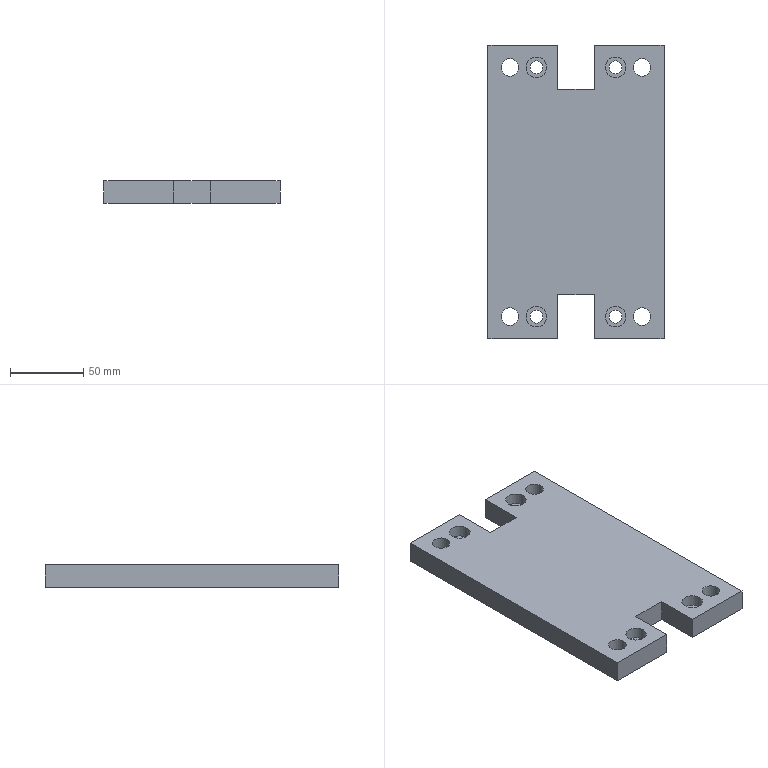Part | STEP file | 冲床-300配套压波_id854_x_t | 1 solid | 30 faces | box 120 x 200 x 15 mm | volume 324088 mm3 | plane 18 | cylinder 12 | commonest cylinder face diameters 8.7 x4 12 x4 14 x4
STEP:
#1=CARTESIAN_POINT('',(1785.,85.,60.));
#2=VERTEX_POINT('',#1);
#3=CARTESIAN_POINT('',(1778.,85.,60.));
#4=DIRECTION('',(0.,0.,-1.));
#5=DIRECTION('',(1.,0.,0.));
#6=AXIS2_PLACEMENT_3D('',#3,#4,#5);
#7=CIRCLE('',#6,7.);
#8=EDGE_CURVE('',#2,#2,#7,.T.);
#9=ORIENTED_EDGE('',*,*,#8,.F.);
#10=EDGE_LOOP('',(#9));
#11=FACE_BOUND('',#10,.T.);
#12=CARTESIAN_POINT('',(1782.35,85.,60.));
#13=VERTEX_POINT('',#12);
#14=CARTESIAN_POINT('',(1778.,85.,60.));
#15=DIRECTION('',(0.,0.,-1.));
#16=DIRECTION('',(1.,0.,0.));
#17=AXIS2_PLACEMENT_3D('',#14,#15,#16);
#18=CIRCLE('',#17,4.35);
#19=EDGE_CURVE('',#13,#13,#18,.T.);
#20=ORIENTED_EDGE('',*,*,#19,.T.);
#21=EDGE_LOOP('',(#20));
#22=FACE_BOUND('',#21,.T.);
#23=CARTESIAN_POINT('',(1778.,85.,60.));
#24=DIRECTION('',(0.,0.,1.));
#25=DIRECTION('',(1.,0.,0.));
#26=AXIS2_PLACEMENT_3D('',#23,#24,#25);
#27=PLANE('',#26);
#28=ADVANCED_FACE('',(#11,#22),#27,.T.);
#29=CARTESIAN_POINT('',(1782.35,85.,53.));
#30=VERTEX_POINT('',#29);
#31=CARTESIAN_POINT('',(1778.,85.,53.));
#32=DIRECTION('',(0.,0.,1.));
#33=DIRECTION('',(1.,0.,0.));
#34=AXIS2_PLACEMENT_3D('',#31,#32,#33);
#35=CIRCLE('',#34,4.35);
#36=EDGE_CURVE('',#30,#30,#35,.T.);
#37=ORIENTED_EDGE('',*,*,#36,.F.);
#38=EDGE_LOOP('',(#37));
#39=FACE_BOUND('',#38,.T.);
#40=ORIENTED_EDGE('',*,*,#19,.F.);
#41=EDGE_LOOP('',(#40));
#42=FACE_BOUND('',#41,.T.);
#43=CARTESIAN_POINT('',(1778.,85.,87.));
#44=DIRECTION('',(0.,0.,-1.));
#45=DIRECTION('',(-1.,0.,0.));
#46=AXIS2_PLACEMENT_3D('',#43,#44,#45);
#47=CYLINDRICAL_SURFACE('',#46,4.35);
#48=ADVANCED_FACE('',(#39,#42),#47,.F.);
#49=ORIENTED_EDGE('',*,*,#8,.T.);
#50=EDGE_LOOP('',(#49));
#51=FACE_BOUND('',#50,.T.);
#52=CARTESIAN_POINT('',(1785.,85.,68.));
#53=VERTEX_POINT('',#52);
#54=CARTESIAN_POINT('',(1778.,85.,68.));
#55=DIRECTION('',(0.,0.,-1.));
#56=DIRECTION('',(1.,0.,0.));
#57=AXIS2_PLACEMENT_3D('',#54,#55,#56);
#58=CIRCLE('',#57,7.);
#59=EDGE_CURVE('',#53,#53,#58,.T.);
#60=ORIENTED_EDGE('',*,*,#59,.F.);
#61=EDGE_LOOP('',(#60));
#62=FACE_BOUND('',#61,.T.);
#63=CARTESIAN_POINT('',(1778.,85.,60.));
#64=DIRECTION('',(0.,0.,1.));
#65=DIRECTION('',(1.,0.,0.));
#66=AXIS2_PLACEMENT_3D('',#63,#64,#65);
#67=CYLINDRICAL_SURFACE('',#66,7.);
#68=ADVANCED_FACE('',(#51,#62),#67,.F.);
#69=CARTESIAN_POINT('',(1785.,-85.,60.));
#70=VERTEX_POINT('',#69);
#71=CARTESIAN_POINT('',(1778.,-85.,60.));
#72=DIRECTION('',(0.,0.,-1.));
#73=DIRECTION('',(1.,0.,0.));
#74=AXIS2_PLACEMENT_3D('',#71,#72,#73);
#75=CIRCLE('',#74,7.);
#76=EDGE_CURVE('',#70,#70,#75,.T.);
#77=ORIENTED_EDGE('',*,*,#76,.F.);
#78=EDGE_LOOP('',(#77));
#79=FACE_BOUND('',#78,.T.);
#80=CARTESIAN_POINT('',(1782.35,-85.,60.));
#81=VERTEX_POINT('',#80);
#82=CARTESIAN_POINT('',(1778.,-85.,60.));
#83=DIRECTION('',(0.,0.,-1.));
#84=DIRECTION('',(1.,0.,0.));
#85=AXIS2_PLACEMENT_3D('',#82,#83,#84);
#86=CIRCLE('',#85,4.35);
#87=EDGE_CURVE('',#81,#81,#86,.T.);
#88=ORIENTED_EDGE('',*,*,#87,.T.);
#89=EDGE_LOOP('',(#88));
#90=FACE_BOUND('',#89,.T.);
#91=CARTESIAN_POINT('',(1778.,-85.,60.));
#92=DIRECTION('',(0.,0.,1.));
#93=DIRECTION('',(1.,0.,0.));
#94=AXIS2_PLACEMENT_3D('',#91,#92,#93);
#95=PLANE('',#94);
#96=ADVANCED_FACE('',(#79,#90),#95,.T.);
#97=CARTESIAN_POINT('',(1825.,-85.,60.));
#98=VERTEX_POINT('',#97);
#99=CARTESIAN_POINT('',(1832.,-85.,60.));
#100=DIRECTION('',(0.,0.,-1.));
#101=DIRECTION('',(-1.,0.,0.));
#102=AXIS2_PLACEMENT_3D('',#99,#100,#101);
#103=CIRCLE('',#102,7.);
#104=EDGE_CURVE('',#98,#98,#103,.T.);
#105=ORIENTED_EDGE('',*,*,#104,.F.);
#106=EDGE_LOOP('',(#105));
#107=FACE_BOUND('',#106,.T.);
#108=CARTESIAN_POINT('',(1827.65,-85.,60.));
#109=VERTEX_POINT('',#108);
#110=CARTESIAN_POINT('',(1832.,-85.,60.));
#111=DIRECTION('',(0.,0.,-1.));
#112=DIRECTION('',(-1.,0.,0.));
#113=AXIS2_PLACEMENT_3D('',#110,#111,#112);
#114=CIRCLE('',#113,4.35);
#115=EDGE_CURVE('',#109,#109,#114,.T.);
#116=ORIENTED_EDGE('',*,*,#115,.T.);
#117=EDGE_LOOP('',(#116));
#118=FACE_BOUND('',#117,.T.);
#119=CARTESIAN_POINT('',(1832.,-85.,60.));
#120=DIRECTION('',(0.,0.,1.));
#121=DIRECTION('',(-1.,0.,0.));
#122=AXIS2_PLACEMENT_3D('',#119,#120,#121);
#123=PLANE('',#122);
#124=ADVANCED_FACE('',(#107,#118),#123,.T.);
#125=CARTESIAN_POINT('',(1856.,-85.,68.));
#126=VERTEX_POINT('',#125);
#127=CARTESIAN_POINT('',(1850.,-85.,68.));
#128=DIRECTION('',(0.,0.,1.));
#129=DIRECTION('',(1.,0.,0.));
#130=AXIS2_PLACEMENT_3D('',#127,#128,#129);
#131=CIRCLE('',#130,6.);
#132=EDGE_CURVE('',#126,#126,#131,.T.);
#133=ORIENTED_EDGE('',*,*,#132,.T.);
#134=EDGE_LOOP('',(#133));
#135=FACE_BOUND('',#134,.T.);
#136=CARTESIAN_POINT('',(1856.,-85.,53.));
#137=VERTEX_POINT('',#136);
#138=CARTESIAN_POINT('',(1850.,-85.,53.));
#139=DIRECTION('',(0.,0.,1.));
#140=DIRECTION('',(1.,0.,0.));
#141=AXIS2_PLACEMENT_3D('',#138,#139,#140);
#142=CIRCLE('',#141,6.);
#143=EDGE_CURVE('',#137,#137,#142,.T.);
#144=ORIENTED_EDGE('',*,*,#143,.F.);
#145=EDGE_LOOP('',(#144));
#146=FACE_BOUND('',#145,.T.);
#147=CARTESIAN_POINT('',(1850.,-85.,-78.5));
#148=DIRECTION('',(0.,0.,1.));
#149=DIRECTION('',(1.,0.,0.));
#150=AXIS2_PLACEMENT_3D('',#147,#148,#149);
#151=CYLINDRICAL_SURFACE('',#150,6.);
#152=ADVANCED_FACE('',(#135,#146),#151,.F.);
#153=CARTESIAN_POINT('',(1766.,-85.,68.));
#154=VERTEX_POINT('',#153);
#155=CARTESIAN_POINT('',(1760.,-85.,68.));
#156=DIRECTION('',(0.,0.,1.));
#157=DIRECTION('',(1.,0.,0.));
#158=AXIS2_PLACEMENT_3D('',#155,#156,#157);
#159=CIRCLE('',#158,6.);
#160=EDGE_CURVE('',#154,#154,#159,.T.);
#161=ORIENTED_EDGE('',*,*,#160,.T.);
#162=EDGE_LOOP('',(#161));
#163=FACE_BOUND('',#162,.T.);
#164=CARTESIAN_POINT('',(1766.,-85.,53.));
#165=VERTEX_POINT('',#164);
#166=CARTESIAN_POINT('',(1760.,-85.,53.));
#167=DIRECTION('',(0.,0.,1.));
#168=DIRECTION('',(1.,0.,0.));
#169=AXIS2_PLACEMENT_3D('',#166,#167,#168);
#170=CIRCLE('',#169,6.);
#171=EDGE_CURVE('',#165,#165,#170,.T.);
#172=ORIENTED_EDGE('',*,*,#171,.F.);
#173=EDGE_LOOP('',(#172));
#174=FACE_BOUND('',#173,.T.);
#175=CARTESIAN_POINT('',(1760.,-85.,-78.5));
#176=DIRECTION('',(0.,0.,1.));
#177=DIRECTION('',(1.,0.,0.));
#178=AXIS2_PLACEMENT_3D('',#175,#176,#177);
#179=CYLINDRICAL_SURFACE('',#178,6.);
#180=ADVANCED_FACE('',(#163,#174),#179,.F.);
#181=CARTESIAN_POINT('',(1856.,85.,68.));
#182=VERTEX_POINT('',#181);
#183=CARTESIAN_POINT('',(1850.,85.,68.));
#184=DIRECTION('',(0.,0.,1.));
#185=DIRECTION('',(1.,0.,0.));
#186=AXIS2_PLACEMENT_3D('',#183,#184,#185);
#187=CIRCLE('',#186,6.);
#188=EDGE_CURVE('',#182,#182,#187,.T.);
#189=ORIENTED_EDGE('',*,*,#188,.T.);
#190=EDGE_LOOP('',(#189));
#191=FACE_BOUND('',#190,.T.);
#192=CARTESIAN_POINT('',(1856.,85.,53.));
#193=VERTEX_POINT('',#192);
#194=CARTESIAN_POINT('',(1850.,85.,53.));
#195=DIRECTION('',(0.,0.,1.));
#196=DIRECTION('',(1.,0.,0.));
#197=AXIS2_PLACEMENT_3D('',#194,#195,#196);
#198=CIRCLE('',#197,6.);
#199=EDGE_CURVE('',#193,#193,#198,.T.);
#200=ORIENTED_EDGE('',*,*,#199,.F.);
#201=EDGE_LOOP('',(#200));
#202=FACE_BOUND('',#201,.T.);
#203=CARTESIAN_POINT('',(1850.,85.,-78.5));
#204=DIRECTION('',(0.,0.,1.));
#205=DIRECTION('',(1.,0.,0.));
#206=AXIS2_PLACEMENT_3D('',#203,#204,#205);
#207=CYLINDRICAL_SURFACE('',#206,6.);
#208=ADVANCED_FACE('',(#191,#202),#207,.F.);
#209=CARTESIAN_POINT('',(1766.,85.,68.));
#210=VERTEX_POINT('',#209);
#211=CARTESIAN_POINT('',(1760.,85.,68.));
#212=DIRECTION('',(0.,0.,1.));
#213=DIRECTION('',(1.,0.,0.));
#214=AXIS2_PLACEMENT_3D('',#211,#212,#213);
#215=CIRCLE('',#214,6.);
#216=EDGE_CURVE('',#210,#210,#215,.T.);
#217=ORIENTED_EDGE('',*,*,#216,.T.);
#218=EDGE_LOOP('',(#217));
#219=FACE_BOUND('',#218,.T.);
#220=CARTESIAN_POINT('',(1766.,85.,53.));
#221=VERTEX_POINT('',#220);
#222=CARTESIAN_POINT('',(1760.,85.,53.));
#223=DIRECTION('',(0.,0.,1.));
#224=DIRECTION('',(1.,0.,0.));
#225=AXIS2_PLACEMENT_3D('',#222,#223,#224);
#226=CIRCLE('',#225,6.);
#227=EDGE_CURVE('',#221,#221,#226,.T.);
#228=ORIENTED_EDGE('',*,*,#227,.F.);
#229=EDGE_LOOP('',(#228));
#230=FACE_BOUND('',#229,.T.);
#231=CARTESIAN_POINT('',(1760.,85.,-78.5));
#232=DIRECTION('',(0.,0.,1.));
#233=DIRECTION('',(1.,0.,0.));
#234=AXIS2_PLACEMENT_3D('',#231,#232,#233);
#235=CYLINDRICAL_SURFACE('',#234,6.);
#236=ADVANCED_FACE('',(#219,#230),#235,.F.);
#237=CARTESIAN_POINT('',(1817.52,70.,68.));
#238=VERTEX_POINT('',#237);
#239=CARTESIAN_POINT('',(1817.52,70.,53.));
#240=VERTEX_POINT('',#239);
#241=CARTESIAN_POINT('',(1817.52,70.,68.));
#242=DIRECTION('',(0.,0.,-1.));
#243=VECTOR('',#242,1.);
#244=LINE('',#241,#243);
#245=EDGE_CURVE('',#238,#240,#244,.T.);
#246=ORIENTED_EDGE('',*,*,#245,.F.);
#247=CARTESIAN_POINT('',(1817.52,100.,68.));
#248=VERTEX_POINT('',#247);
#249=CARTESIAN_POINT('',(1817.52,58.462,68.));
#250=DIRECTION('',(0.,1.,0.));
#251=VECTOR('',#250,1.);
#252=LINE('',#249,#251);
#253=EDGE_CURVE('',#238,#248,#252,.T.);
#254=ORIENTED_EDGE('',*,*,#253,.T.);
#255=CARTESIAN_POINT('',(1817.52,100.,53.));
#256=VERTEX_POINT('',#255);
#257=CARTESIAN_POINT('',(1817.52,100.,68.));
#258=DIRECTION('',(0.,0.,-1.));
#259=VECTOR('',#258,1.);
#260=LINE('',#257,#259);
#261=EDGE_CURVE('',#248,#256,#260,.T.);
#262=ORIENTED_EDGE('',*,*,#261,.T.);
#263=CARTESIAN_POINT('',(1817.52,58.462,53.));
#264=DIRECTION('',(0.,1.,0.));
#265=VECTOR('',#264,1.);
#266=LINE('',#263,#265);
#267=EDGE_CURVE('',#240,#256,#266,.T.);
#268=ORIENTED_EDGE('',*,*,#267,.F.);
#269=EDGE_LOOP('',(#246,#254,#262,#268));
#270=FACE_OUTER_BOUND('',#269,.T.);
#271=CARTESIAN_POINT('',(1817.52,58.462,68.));
#272=DIRECTION('',(-1.,0.,0.));
#273=DIRECTION('',(0.,0.,1.));
#274=AXIS2_PLACEMENT_3D('',#271,#272,#273);
#275=PLANE('',#274);
#276=ADVANCED_FACE('',(#270),#275,.T.);
#277=CARTESIAN_POINT('',(1792.48,70.,53.));
#278=VERTEX_POINT('',#277);
#279=CARTESIAN_POINT('',(1730.,70.,53.));
#280=DIRECTION('',(-1.,0.,0.));
#281=VECTOR('',#280,1.);
#282=LINE('',#279,#281);
#283=EDGE_CURVE('',#240,#278,#282,.T.);
#284=ORIENTED_EDGE('',*,*,#283,.T.);
#285=CARTESIAN_POINT('',(1792.48,70.,68.));
#286=VERTEX_POINT('',#285);
#287=CARTESIAN_POINT('',(1792.48,70.,68.));
#288=DIRECTION('',(0.,0.,1.));
#289=VECTOR('',#288,1.);
#290=LINE('',#287,#289);
#291=EDGE_CURVE('',#278,#286,#290,.T.);
#292=ORIENTED_EDGE('',*,*,#291,.T.);
#293=CARTESIAN_POINT('',(1730.,70.,68.));
#294=DIRECTION('',(1.,0.,0.));
#295=VECTOR('',#294,1.);
#296=LINE('',#293,#295);
#297=EDGE_CURVE('',#286,#238,#296,.T.);
#298=ORIENTED_EDGE('',*,*,#297,.T.);
#299=ORIENTED_EDGE('',*,*,#245,.T.);
#300=EDGE_LOOP('',(#284,#292,#298,#299));
#301=FACE_OUTER_BOUND('',#300,.T.);
#302=CARTESIAN_POINT('',(1730.,70.,73.));
#303=DIRECTION('',(0.,1.,0.));
#304=DIRECTION('',(-1.,0.,0.));
#305=AXIS2_PLACEMENT_3D('',#302,#303,#304);
#306=PLANE('',#305);
#307=ADVANCED_FACE('',(#301),#306,.T.);
#308=ORIENTED_EDGE('',*,*,#291,.F.);
#309=CARTESIAN_POINT('',(1792.48,100.,53.));
#310=VERTEX_POINT('',#309);
#311=CARTESIAN_POINT('',(1792.48,100.,53.));
#312=DIRECTION('',(0.,-1.,0.));
#313=VECTOR('',#312,1.);
#314=LINE('',#311,#313);
#315=EDGE_CURVE('',#310,#278,#314,.T.);
#316=ORIENTED_EDGE('',*,*,#315,.F.);
#317=CARTESIAN_POINT('',(1792.48,100.,68.));
#318=VERTEX_POINT('',#317);
#319=CARTESIAN_POINT('',(1792.48,100.,68.));
#320=DIRECTION('',(0.,0.,-1.));
#321=VECTOR('',#320,1.);
#322=LINE('',#319,#321);
#323=EDGE_CURVE('',#318,#310,#322,.T.);
#324=ORIENTED_EDGE('',*,*,#323,.F.);
#325=CARTESIAN_POINT('',(1792.48,100.,68.));
#326=DIRECTION('',(0.,-1.,0.));
#327=VECTOR('',#326,1.);
#328=LINE('',#325,#327);
#329=EDGE_CURVE('',#318,#286,#328,.T.);
#330=ORIENTED_EDGE('',*,*,#329,.T.);
#331=EDGE_LOOP('',(#308,#316,#324,#330));
#332=FACE_OUTER_BOUND('',#331,.T.);
#333=CARTESIAN_POINT('',(1792.48,100.,68.));
#334=DIRECTION('',(1.,0.,0.));
#335=DIRECTION('',(0.,0.,-1.));
#336=AXIS2_PLACEMENT_3D('',#333,#334,#335);
#337=PLANE('',#336);
#338=ADVANCED_FACE('',(#332),#337,.T.);
#339=CARTESIAN_POINT('',(1745.,100.,68.));
#340=VERTEX_POINT('',#339);
#341=CARTESIAN_POINT('',(1730.,100.,68.));
#342=DIRECTION('',(1.,0.,0.));
#343=VECTOR('',#342,1.);
#344=LINE('',#341,#343);
#345=EDGE_CURVE('',#340,#318,#344,.T.);
#346=ORIENTED_EDGE('',*,*,#345,.T.);
#347=ORIENTED_EDGE('',*,*,#323,.T.);
#348=CARTESIAN_POINT('',(1745.,100.,53.));
#349=VERTEX_POINT('',#348);
#350=CARTESIAN_POINT('',(1730.,100.,53.));
#351=DIRECTION('',(1.,0.,0.));
#352=VECTOR('',#351,1.);
#353=LINE('',#350,#352);
#354=EDGE_CURVE('',#349,#310,#353,.T.);
#355=ORIENTED_EDGE('',*,*,#354,.F.);
#356=CARTESIAN_POINT('',(1745.,100.,68.));
#357=DIRECTION('',(0.,0.,-1.));
#358=VECTOR('',#357,1.);
#359=LINE('',#356,#358);
#360=EDGE_CURVE('',#340,#349,#359,.T.);
#361=ORIENTED_EDGE('',*,*,#360,.F.);
#362=EDGE_LOOP('',(#346,#347,#355,#361));
#363=FACE_OUTER_BOUND('',#362,.T.);
#364=CARTESIAN_POINT('',(1730.,100.,68.));
#365=DIRECTION('',(0.,-1.,0.));
#366=DIRECTION('',(1.,0.,0.));
#367=AXIS2_PLACEMENT_3D('',#364,#365,#366);
#368=PLANE('',#367);
#369=ADVANCED_FACE('',(#363),#368,.F.);
#370=CARTESIAN_POINT('',(1745.,-100.,53.));
#371=VERTEX_POINT('',#370);
#372=CARTESIAN_POINT('',(1745.,-60.,53.));
#373=DIRECTION('',(0.,1.,0.));
#374=VECTOR('',#373,1.);
#375=LINE('',#372,#374);
#376=EDGE_CURVE('',#371,#349,#375,.T.);
#377=ORIENTED_EDGE('',*,*,#376,.F.);
#378=CARTESIAN_POINT('',(1745.,-100.,68.));
#379=VERTEX_POINT('',#378);
#380=CARTESIAN_POINT('',(1745.,-100.,68.));
#381=DIRECTION('',(0.,0.,1.));
#382=VECTOR('',#381,1.);
#383=LINE('',#380,#382);
#384=EDGE_CURVE('',#371,#379,#383,.T.);
#385=ORIENTED_EDGE('',*,*,#384,.T.);
#386=CARTESIAN_POINT('',(1745.,-60.,68.));
#387=DIRECTION('',(0.,1.,0.));
#388=VECTOR('',#387,1.);
#389=LINE('',#386,#388);
#390=EDGE_CURVE('',#379,#340,#389,.T.);
#391=ORIENTED_EDGE('',*,*,#390,.T.);
#392=ORIENTED_EDGE('',*,*,#360,.T.);
#393=EDGE_LOOP('',(#377,#385,#391,#392));
#394=FACE_OUTER_BOUND('',#393,.T.);
#395=CARTESIAN_POINT('',(1745.,-60.,68.));
#396=DIRECTION('',(-1.,0.,0.));
#397=DIRECTION('',(0.,0.,1.));
#398=AXIS2_PLACEMENT_3D('',#395,#396,#397);
#399=PLANE('',#398);
#400=ADVANCED_FACE('',(#394),#399,.T.);
#401=CARTESIAN_POINT('',(1792.48,-100.,68.));
#402=VERTEX_POINT('',#401);
#403=CARTESIAN_POINT('',(1730.,-100.,68.));
#404=DIRECTION('',(-1.,0.,0.));
#405=VECTOR('',#404,1.);
#406=LINE('',#403,#405);
#407=EDGE_CURVE('',#402,#379,#406,.T.);
#408=ORIENTED_EDGE('',*,*,#407,.T.);
#409=ORIENTED_EDGE('',*,*,#384,.F.);
#410=CARTESIAN_POINT('',(1792.48,-100.,53.));
#411=VERTEX_POINT('',#410);
#412=CARTESIAN_POINT('',(1730.,-100.,53.));
#413=DIRECTION('',(-1.,0.,0.));
#414=VECTOR('',#413,1.);
#415=LINE('',#412,#414);
#416=EDGE_CURVE('',#411,#371,#415,.T.);
#417=ORIENTED_EDGE('',*,*,#416,.F.);
#418=CARTESIAN_POINT('',(1792.48,-100.,68.));
#419=DIRECTION('',(0.,0.,1.));
#420=VECTOR('',#419,1.);
#421=LINE('',#418,#420);
#422=EDGE_CURVE('',#411,#402,#421,.T.);
#423=ORIENTED_EDGE('',*,*,#422,.T.);
#424=EDGE_LOOP('',(#408,#409,#417,#423));
#425=FACE_OUTER_BOUND('',#424,.T.);
#426=CARTESIAN_POINT('',(1730.,-100.,68.));
#427=DIRECTION('',(0.,1.,0.));
#428=DIRECTION('',(1.,0.,0.));
#429=AXIS2_PLACEMENT_3D('',#426,#427,#428);
#430=PLANE('',#429);
#431=ADVANCED_FACE('',(#425),#430,.F.);
#432=CARTESIAN_POINT('',(1792.48,-70.,53.));
#433=VERTEX_POINT('',#432);
#434=CARTESIAN_POINT('',(1792.48,-100.,53.));
#435=DIRECTION('',(0.,-1.,0.));
#436=VECTOR('',#435,1.);
#437=LINE('',#434,#436);
#438=EDGE_CURVE('',#433,#411,#437,.T.);
#439=ORIENTED_EDGE('',*,*,#438,.F.);
#440=CARTESIAN_POINT('',(1792.48,-70.,68.));
#441=VERTEX_POINT('',#440);
#442=CARTESIAN_POINT('',(1792.48,-70.,150.));
#443=DIRECTION('',(0.,0.,1.));
#444=VECTOR('',#443,1.);
#445=LINE('',#442,#444);
#446=EDGE_CURVE('',#433,#441,#445,.T.);
#447=ORIENTED_EDGE('',*,*,#446,.T.);
#448=CARTESIAN_POINT('',(1792.48,-100.,68.));
#449=DIRECTION('',(0.,-1.,0.));
#450=VECTOR('',#449,1.);
#451=LINE('',#448,#450);
#452=EDGE_CURVE('',#441,#402,#451,.T.);
#453=ORIENTED_EDGE('',*,*,#452,.T.);
#454=ORIENTED_EDGE('',*,*,#422,.F.);
#455=EDGE_LOOP('',(#439,#447,#453,#454));
#456=FACE_OUTER_BOUND('',#455,.T.);
#457=CARTESIAN_POINT('',(1792.48,-100.,68.));
#458=DIRECTION('',(1.,0.,0.));
#459=DIRECTION('',(0.,0.,-1.));
#460=AXIS2_PLACEMENT_3D('',#457,#458,#459);
#461=PLANE('',#460);
#462=ADVANCED_FACE('',(#456),#461,.T.);
#463=CARTESIAN_POINT('',(1817.52,-70.,53.));
#464=VERTEX_POINT('',#463);
#465=CARTESIAN_POINT('',(1730.,-70.,53.));
#466=DIRECTION('',(1.,0.,0.));
#467=VECTOR('',#466,1.);
#468=LINE('',#465,#467);
#469=EDGE_CURVE('',#433,#464,#468,.T.);
#470=ORIENTED_EDGE('',*,*,#469,.T.);
#471=CARTESIAN_POINT('',(1817.52,-70.,68.));
#472=VERTEX_POINT('',#471);
#473=CARTESIAN_POINT('',(1817.52,-70.,150.));
#474=DIRECTION('',(0.,0.,-1.));
#475=VECTOR('',#474,1.);
#476=LINE('',#473,#475);
#477=EDGE_CURVE('',#472,#464,#476,.T.);
#478=ORIENTED_EDGE('',*,*,#477,.F.);
#479=CARTESIAN_POINT('',(1730.,-70.,68.));
#480=DIRECTION('',(-1.,0.,0.));
#481=VECTOR('',#480,1.);
#482=LINE('',#479,#481);
#483=EDGE_CURVE('',#472,#441,#482,.T.);
#484=ORIENTED_EDGE('',*,*,#483,.T.);
#485=ORIENTED_EDGE('',*,*,#446,.F.);
#486=EDGE_LOOP('',(#470,#478,#484,#485));
#487=FACE_OUTER_BOUND('',#486,.T.);
#488=CARTESIAN_POINT('',(1730.,-70.,150.));
#489=DIRECTION('',(0.,-1.,0.));
#490=DIRECTION('',(-1.,0.,0.));
#491=AXIS2_PLACEMENT_3D('',#488,#489,#490);
#492=PLANE('',#491);
#493=ADVANCED_FACE('',(#487),#492,.T.);
#494=CARTESIAN_POINT('',(1817.52,-100.,53.));
#495=VERTEX_POINT('',#494);
#496=CARTESIAN_POINT('',(1817.52,-100.,68.));
#497=VERTEX_POINT('',#496);
#498=CARTESIAN_POINT('',(1817.52,-100.,68.));
#499=DIRECTION('',(0.,0.,1.));
#500=VECTOR('',#499,1.);
#501=LINE('',#498,#500);
#502=EDGE_CURVE('',#495,#497,#501,.T.);
#503=ORIENTED_EDGE('',*,*,#502,.T.);
#504=CARTESIAN_POINT('',(1817.52,-58.462,68.));
#505=DIRECTION('',(0.,1.,0.));
#506=VECTOR('',#505,1.);
#507=LINE('',#504,#506);
#508=EDGE_CURVE('',#497,#472,#507,.T.);
#509=ORIENTED_EDGE('',*,*,#508,.T.);
#510=ORIENTED_EDGE('',*,*,#477,.T.);
#511=CARTESIAN_POINT('',(1817.52,-58.462,53.));
#512=DIRECTION('',(0.,1.,0.));
#513=VECTOR('',#512,1.);
#514=LINE('',#511,#513);
#515=EDGE_CURVE('',#495,#464,#514,.T.);
#516=ORIENTED_EDGE('',*,*,#515,.F.);
#517=EDGE_LOOP('',(#503,#509,#510,#516));
#518=FACE_OUTER_BOUND('',#517,.T.);
#519=CARTESIAN_POINT('',(1817.52,-58.462,68.));
#520=DIRECTION('',(-1.,0.,0.));
#521=DIRECTION('',(0.,0.,1.));
#522=AXIS2_PLACEMENT_3D('',#519,#520,#521);
#523=PLANE('',#522);
#524=ADVANCED_FACE('',(#518),#523,.T.);
#525=ORIENTED_EDGE('',*,*,#502,.F.);
#526=CARTESIAN_POINT('',(1865.,-100.,53.));
#527=VERTEX_POINT('',#526);
#528=CARTESIAN_POINT('',(1730.,-100.,53.));
#529=DIRECTION('',(-1.,0.,0.));
#530=VECTOR('',#529,1.);
#531=LINE('',#528,#530);
#532=EDGE_CURVE('',#527,#495,#531,.T.);
#533=ORIENTED_EDGE('',*,*,#532,.F.);
#534=CARTESIAN_POINT('',(1865.,-100.,68.));
#535=VERTEX_POINT('',#534);
#536=CARTESIAN_POINT('',(1865.,-100.,68.));
#537=DIRECTION('',(0.,0.,1.));
#538=VECTOR('',#537,1.);
#539=LINE('',#536,#538);
#540=EDGE_CURVE('',#527,#535,#539,.T.);
#541=ORIENTED_EDGE('',*,*,#540,.T.);
#542=CARTESIAN_POINT('',(1730.,-100.,68.));
#543=DIRECTION('',(-1.,0.,0.));
#544=VECTOR('',#543,1.);
#545=LINE('',#542,#544);
#546=EDGE_CURVE('',#535,#497,#545,.T.);
#547=ORIENTED_EDGE('',*,*,#546,.T.);
#548=EDGE_LOOP('',(#525,#533,#541,#547));
#549=FACE_OUTER_BOUND('',#548,.T.);
#550=CARTESIAN_POINT('',(1730.,-100.,68.));
#551=DIRECTION('',(0.,1.,0.));
#552=DIRECTION('',(1.,0.,0.));
#553=AXIS2_PLACEMENT_3D('',#550,#551,#552);
#554=PLANE('',#553);
#555=ADVANCED_FACE('',(#549),#554,.F.);
#556=CARTESIAN_POINT('',(1865.,100.,68.));
#557=VERTEX_POINT('',#556);
#558=CARTESIAN_POINT('',(1865.,80.,68.));
#559=DIRECTION('',(0.,1.,0.));
#560=VECTOR('',#559,1.);
#561=LINE('',#558,#560);
#562=EDGE_CURVE('',#535,#557,#561,.T.);
#563=ORIENTED_EDGE('',*,*,#562,.F.);
#564=ORIENTED_EDGE('',*,*,#540,.F.);
#565=CARTESIAN_POINT('',(1865.,100.,53.));
#566=VERTEX_POINT('',#565);
#567=CARTESIAN_POINT('',(1865.,80.,53.));
#568=DIRECTION('',(0.,1.,0.));
#569=VECTOR('',#568,1.);
#570=LINE('',#567,#569);
#571=EDGE_CURVE('',#527,#566,#570,.T.);
#572=ORIENTED_EDGE('',*,*,#571,.T.);
#573=CARTESIAN_POINT('',(1865.,100.,68.));
#574=DIRECTION('',(0.,0.,-1.));
#575=VECTOR('',#574,1.);
#576=LINE('',#573,#575);
#577=EDGE_CURVE('',#557,#566,#576,.T.);
#578=ORIENTED_EDGE('',*,*,#577,.F.);
#579=EDGE_LOOP('',(#563,#564,#572,#578));
#580=FACE_OUTER_BOUND('',#579,.T.);
#581=CARTESIAN_POINT('',(1865.,60.,68.));
#582=DIRECTION('',(1.,0.,0.));
#583=DIRECTION('',(0.,0.,-1.));
#584=AXIS2_PLACEMENT_3D('',#581,#582,#583);
#585=PLANE('',#584);
#586=ADVANCED_FACE('',(#580),#585,.T.);
#587=ORIENTED_EDGE('',*,*,#261,.F.);
#588=CARTESIAN_POINT('',(1730.,100.,68.));
#589=DIRECTION('',(1.,0.,0.));
#590=VECTOR('',#589,1.);
#591=LINE('',#588,#590);
#592=EDGE_CURVE('',#248,#557,#591,.T.);
#593=ORIENTED_EDGE('',*,*,#592,.T.);
#594=ORIENTED_EDGE('',*,*,#577,.T.);
#595=CARTESIAN_POINT('',(1730.,100.,53.));
#596=DIRECTION('',(1.,0.,0.));
#597=VECTOR('',#596,1.);
#598=LINE('',#595,#597);
#599=EDGE_CURVE('',#256,#566,#598,.T.);
#600=ORIENTED_EDGE('',*,*,#599,.F.);
#601=EDGE_LOOP('',(#587,#593,#594,#600));
#602=FACE_OUTER_BOUND('',#601,.T.);
#603=CARTESIAN_POINT('',(1730.,100.,68.));
#604=DIRECTION('',(0.,-1.,0.));
#605=DIRECTION('',(1.,0.,0.));
#606=AXIS2_PLACEMENT_3D('',#603,#604,#605);
#607=PLANE('',#606);
#608=ADVANCED_FACE('',(#602),#607,.F.);
#609=CARTESIAN_POINT('',(1782.35,-85.,53.));
#610=VERTEX_POINT('',#609);
#611=CARTESIAN_POINT('',(1778.,-85.,53.));
#612=DIRECTION('',(0.,0.,1.));
#613=DIRECTION('',(1.,0.,0.));
#614=AXIS2_PLACEMENT_3D('',#611,#612,#613);
#615=CIRCLE('',#614,4.35);
#616=EDGE_CURVE('',#610,#610,#615,.T.);
#617=ORIENTED_EDGE('',*,*,#616,.F.);
#618=EDGE_LOOP('',(#617));
#619=FACE_BOUND('',#618,.T.);
#620=ORIENTED_EDGE('',*,*,#87,.F.);
#621=EDGE_LOOP('',(#620));
#622=FACE_BOUND('',#621,.T.);
#623=CARTESIAN_POINT('',(1778.,-85.,87.));
#624=DIRECTION('',(0.,0.,-1.));
#625=DIRECTION('',(-1.,0.,0.));
#626=AXIS2_PLACEMENT_3D('',#623,#624,#625);
#627=CYLINDRICAL_SURFACE('',#626,4.35);
#628=ADVANCED_FACE('',(#619,#622),#627,.F.);
#629=CARTESIAN_POINT('',(1827.65,-85.,53.));
#630=VERTEX_POINT('',#629);
#631=CARTESIAN_POINT('',(1832.,-85.,53.));
#632=DIRECTION('',(0.,0.,1.));
#633=DIRECTION('',(-1.,0.,0.));
#634=AXIS2_PLACEMENT_3D('',#631,#632,#633);
#635=CIRCLE('',#634,4.35);
#636=EDGE_CURVE('',#630,#630,#635,.T.);
#637=ORIENTED_EDGE('',*,*,#636,.F.);
#638=EDGE_LOOP('',(#637));
#639=FACE_BOUND('',#638,.T.);
#640=ORIENTED_EDGE('',*,*,#115,.F.);
#641=EDGE_LOOP('',(#640));
#642=FACE_BOUND('',#641,.T.);
#643=CARTESIAN_POINT('',(1832.,-85.,87.));
#644=DIRECTION('',(0.,0.,-1.));
#645=DIRECTION('',(1.,0.,0.));
#646=AXIS2_PLACEMENT_3D('',#643,#644,#645);
#647=CYLINDRICAL_SURFACE('',#646,4.35);
#648=ADVANCED_FACE('',(#639,#642),#647,.F.);
#649=CARTESIAN_POINT('',(1827.65,85.,53.));
#650=VERTEX_POINT('',#649);
#651=CARTESIAN_POINT('',(1832.,85.,53.));
#652=DIRECTION('',(0.,0.,1.));
#653=DIRECTION('',(-1.,0.,0.));
#654=AXIS2_PLACEMENT_3D('',#651,#652,#653);
#655=CIRCLE('',#654,4.35);
#656=EDGE_CURVE('',#650,#650,#655,.T.);
#657=ORIENTED_EDGE('',*,*,#656,.T.);
#658=EDGE_LOOP('',(#657));
#659=FACE_BOUND('',#658,.T.);
#660=ORIENTED_EDGE('',*,*,#36,.T.);
#661=EDGE_LOOP('',(#660));
#662=FACE_BOUND('',#661,.T.);
#663=ORIENTED_EDGE('',*,*,#636,.T.);
#664=EDGE_LOOP('',(#663));
#665=FACE_BOUND('',#664,.T.);
#666=ORIENTED_EDGE('',*,*,#616,.T.);
#667=EDGE_LOOP('',(#666));
#668=FACE_BOUND('',#667,.T.);
#669=ORIENTED_EDGE('',*,*,#599,.T.);
#670=ORIENTED_EDGE('',*,*,#571,.F.);
#671=ORIENTED_EDGE('',*,*,#532,.T.);
#672=ORIENTED_EDGE('',*,*,#515,.T.);
#673=ORIENTED_EDGE('',*,*,#469,.F.);
#674=ORIENTED_EDGE('',*,*,#438,.T.);
#675=ORIENTED_EDGE('',*,*,#416,.T.);
#676=ORIENTED_EDGE('',*,*,#376,.T.);
#677=ORIENTED_EDGE('',*,*,#354,.T.);
#678=ORIENTED_EDGE('',*,*,#315,.T.);
#679=ORIENTED_EDGE('',*,*,#283,.F.);
#680=ORIENTED_EDGE('',*,*,#267,.T.);
#681=EDGE_LOOP('',(#669,#670,#671,#672,#673,#674,#675,#676,#677,#678,#679,#680));
#682=FACE_BOUND('',#681,.T.);
#683=ORIENTED_EDGE('',*,*,#227,.T.);
#684=EDGE_LOOP('',(#683));
#685=FACE_BOUND('',#684,.T.);
#686=ORIENTED_EDGE('',*,*,#199,.T.);
#687=EDGE_LOOP('',(#686));
#688=FACE_BOUND('',#687,.T.);
#689=ORIENTED_EDGE('',*,*,#171,.T.);
#690=EDGE_LOOP('',(#689));
#691=FACE_BOUND('',#690,.T.);
#692=ORIENTED_EDGE('',*,*,#143,.T.);
#693=EDGE_LOOP('',(#692));
#694=FACE_BOUND('',#693,.T.);
#695=CARTESIAN_POINT('',(1730.,80.,53.));
#696=DIRECTION('',(0.,0.,1.));
#697=DIRECTION('',(1.,0.,0.));
#698=AXIS2_PLACEMENT_3D('',#695,#696,#697);
#699=PLANE('',#698);
#700=ADVANCED_FACE('',(#659,#662,#665,#668,#682,#685,#688,#691,#694),#699,.F.);
#701=ORIENTED_EDGE('',*,*,#76,.T.);
#702=EDGE_LOOP('',(#701));
#703=FACE_BOUND('',#702,.T.);
#704=CARTESIAN_POINT('',(1785.,-85.,68.));
#705=VERTEX_POINT('',#704);
#706=CARTESIAN_POINT('',(1778.,-85.,68.));
#707=DIRECTION('',(0.,0.,1.));
#708=DIRECTION('',(1.,0.,0.));
#709=AXIS2_PLACEMENT_3D('',#706,#707,#708);
#710=CIRCLE('',#709,7.);
#711=EDGE_CURVE('',#705,#705,#710,.T.);
#712=ORIENTED_EDGE('',*,*,#711,.T.);
#713=EDGE_LOOP('',(#712));
#714=FACE_BOUND('',#713,.T.);
#715=CARTESIAN_POINT('',(1778.,-85.,60.));
#716=DIRECTION('',(0.,0.,1.));
#717=DIRECTION('',(1.,0.,0.));
#718=AXIS2_PLACEMENT_3D('',#715,#716,#717);
#719=CYLINDRICAL_SURFACE('',#718,7.);
#720=ADVANCED_FACE('',(#703,#714),#719,.F.);
#721=ORIENTED_EDGE('',*,*,#104,.T.);
#722=EDGE_LOOP('',(#721));
#723=FACE_BOUND('',#722,.T.);
#724=CARTESIAN_POINT('',(1825.,-85.,68.));
#725=VERTEX_POINT('',#724);
#726=CARTESIAN_POINT('',(1832.,-85.,68.));
#727=DIRECTION('',(0.,0.,-1.));
#728=DIRECTION('',(-1.,0.,0.));
#729=AXIS2_PLACEMENT_3D('',#726,#727,#728);
#730=CIRCLE('',#729,7.);
#731=EDGE_CURVE('',#725,#725,#730,.T.);
#732=ORIENTED_EDGE('',*,*,#731,.F.);
#733=EDGE_LOOP('',(#732));
#734=FACE_BOUND('',#733,.T.);
#735=CARTESIAN_POINT('',(1832.,-85.,60.));
#736=DIRECTION('',(0.,0.,1.));
#737=DIRECTION('',(-1.,0.,0.));
#738=AXIS2_PLACEMENT_3D('',#735,#736,#737);
#739=CYLINDRICAL_SURFACE('',#738,7.);
#740=ADVANCED_FACE('',(#723,#734),#739,.F.);
#741=CARTESIAN_POINT('',(1825.,85.,68.));
#742=VERTEX_POINT('',#741);
#743=CARTESIAN_POINT('',(1832.,85.,68.));
#744=DIRECTION('',(0.,0.,-1.));
#745=DIRECTION('',(-1.,0.,0.));
#746=AXIS2_PLACEMENT_3D('',#743,#744,#745);
#747=CIRCLE('',#746,7.);
#748=EDGE_CURVE('',#742,#742,#747,.T.);
#749=ORIENTED_EDGE('',*,*,#748,.T.);
#750=EDGE_LOOP('',(#749));
#751=FACE_BOUND('',#750,.T.);
#752=ORIENTED_EDGE('',*,*,#59,.T.);
#753=EDGE_LOOP('',(#752));
#754=FACE_BOUND('',#753,.T.);
#755=ORIENTED_EDGE('',*,*,#731,.T.);
#756=EDGE_LOOP('',(#755));
#757=FACE_BOUND('',#756,.T.);
#758=ORIENTED_EDGE('',*,*,#711,.F.);
#759=EDGE_LOOP('',(#758));
#760=FACE_BOUND('',#759,.T.);
#761=ORIENTED_EDGE('',*,*,#483,.F.);
#762=ORIENTED_EDGE('',*,*,#508,.F.);
#763=ORIENTED_EDGE('',*,*,#546,.F.);
#764=ORIENTED_EDGE('',*,*,#562,.T.);
#765=ORIENTED_EDGE('',*,*,#592,.F.);
#766=ORIENTED_EDGE('',*,*,#253,.F.);
#767=ORIENTED_EDGE('',*,*,#297,.F.);
#768=ORIENTED_EDGE('',*,*,#329,.F.);
#769=ORIENTED_EDGE('',*,*,#345,.F.);
#770=ORIENTED_EDGE('',*,*,#390,.F.);
#771=ORIENTED_EDGE('',*,*,#407,.F.);
#772=ORIENTED_EDGE('',*,*,#452,.F.);
#773=EDGE_LOOP('',(#761,#762,#763,#764,#765,#766,#767,#768,#769,#770,#771,#772));
#774=FACE_BOUND('',#773,.T.);
#775=ORIENTED_EDGE('',*,*,#216,.F.);
#776=EDGE_LOOP('',(#775));
#777=FACE_BOUND('',#776,.T.);
#778=ORIENTED_EDGE('',*,*,#188,.F.);
#779=EDGE_LOOP('',(#778));
#780=FACE_BOUND('',#779,.T.);
#781=ORIENTED_EDGE('',*,*,#132,.F.);
#782=EDGE_LOOP('',(#781));
#783=FACE_BOUND('',#782,.T.);
#784=ORIENTED_EDGE('',*,*,#160,.F.);
#785=EDGE_LOOP('',(#784));
#786=FACE_BOUND('',#785,.T.);
#787=CARTESIAN_POINT('',(1730.,80.,68.));
#788=DIRECTION('',(0.,0.,1.));
#789=DIRECTION('',(1.,0.,0.));
#790=AXIS2_PLACEMENT_3D('',#787,#788,#789);
#791=PLANE('',#790);
#792=ADVANCED_FACE('',(#751,#754,#757,#760,#774,#777,#780,#783,#786),#791,.T.);
#793=CARTESIAN_POINT('',(1825.,85.,60.));
#794=VERTEX_POINT('',#793);
#795=CARTESIAN_POINT('',(1832.,85.,60.));
#796=DIRECTION('',(0.,0.,-1.));
#797=DIRECTION('',(-1.,0.,0.));
#798=AXIS2_PLACEMENT_3D('',#795,#796,#797);
#799=CIRCLE('',#798,7.);
#800=EDGE_CURVE('',#794,#794,#799,.T.);
#801=ORIENTED_EDGE('',*,*,#800,.F.);
#802=EDGE_LOOP('',(#801));
#803=FACE_BOUND('',#802,.T.);
#804=CARTESIAN_POINT('',(1827.65,85.,60.));
#805=VERTEX_POINT('',#804);
#806=CARTESIAN_POINT('',(1832.,85.,60.));
#807=DIRECTION('',(0.,0.,-1.));
#808=DIRECTION('',(-1.,0.,0.));
#809=AXIS2_PLACEMENT_3D('',#806,#807,#808);
#810=CIRCLE('',#809,4.35);
#811=EDGE_CURVE('',#805,#805,#810,.T.);
#812=ORIENTED_EDGE('',*,*,#811,.T.);
#813=EDGE_LOOP('',(#812));
#814=FACE_BOUND('',#813,.T.);
#815=CARTESIAN_POINT('',(1832.,85.,60.));
#816=DIRECTION('',(0.,0.,1.));
#817=DIRECTION('',(-1.,0.,0.));
#818=AXIS2_PLACEMENT_3D('',#815,#816,#817);
#819=PLANE('',#818);
#820=ADVANCED_FACE('',(#803,#814),#819,.T.);
#821=ORIENTED_EDGE('',*,*,#656,.F.);
#822=EDGE_LOOP('',(#821));
#823=FACE_BOUND('',#822,.T.);
#824=ORIENTED_EDGE('',*,*,#811,.F.);
#825=EDGE_LOOP('',(#824));
#826=FACE_BOUND('',#825,.T.);
#827=CARTESIAN_POINT('',(1832.,85.,87.));
#828=DIRECTION('',(0.,0.,-1.));
#829=DIRECTION('',(1.,0.,0.));
#830=AXIS2_PLACEMENT_3D('',#827,#828,#829);
#831=CYLINDRICAL_SURFACE('',#830,4.35);
#832=ADVANCED_FACE('',(#823,#826),#831,.F.);
#833=ORIENTED_EDGE('',*,*,#800,.T.);
#834=EDGE_LOOP('',(#833));
#835=FACE_BOUND('',#834,.T.);
#836=ORIENTED_EDGE('',*,*,#748,.F.);
#837=EDGE_LOOP('',(#836));
#838=FACE_BOUND('',#837,.T.);
#839=CARTESIAN_POINT('',(1832.,85.,60.));
#840=DIRECTION('',(0.,0.,1.));
#841=DIRECTION('',(-1.,0.,0.));
#842=AXIS2_PLACEMENT_3D('',#839,#840,#841);
#843=CYLINDRICAL_SURFACE('',#842,7.);
#844=ADVANCED_FACE('',(#835,#838),#843,.F.);
#845=CLOSED_SHELL('',(#28,#48,#68,#96,#124,#152,#180,#208,#236,#276,#307,#338,#369,#400,#431,#462,#493,#524,#555,#586,#608,#628,#648,#700,#720,#740,#792,#820,#832,#844));
#846=MANIFOLD_SOLID_BREP('',#845);
#847=(LENGTH_UNIT()NAMED_UNIT(*)SI_UNIT(.MILLI.,.METRE.));
#848=UNCERTAINTY_MEASURE_WITH_UNIT(LENGTH_MEASURE(0.00002),#847,'','');
#849=(NAMED_UNIT(*)PLANE_ANGLE_UNIT()SI_UNIT($,.RADIAN.));
#850=PLANE_ANGLE_MEASURE_WITH_UNIT(PLANE_ANGLE_MEASURE(0.01745),#849);
#851=DIMENSIONAL_EXPONENTS(0.,0.,0.,0.,0.,0.,0.);
#852=(CONVERSION_BASED_UNIT('DEGREE',#850)NAMED_UNIT(#851)PLANE_ANGLE_UNIT());
#853=(NAMED_UNIT(*)SI_UNIT($,.STERADIAN.)SOLID_ANGLE_UNIT());
#854=(GEOMETRIC_REPRESENTATION_CONTEXT(3)GLOBAL_UNCERTAINTY_ASSIGNED_CONTEXT((#848))GLOBAL_UNIT_ASSIGNED_CONTEXT((#847,#852,#853))REPRESENTATION_CONTEXT('',''));
#855=ADVANCED_BREP_SHAPE_REPRESENTATION('',(#846),#854);